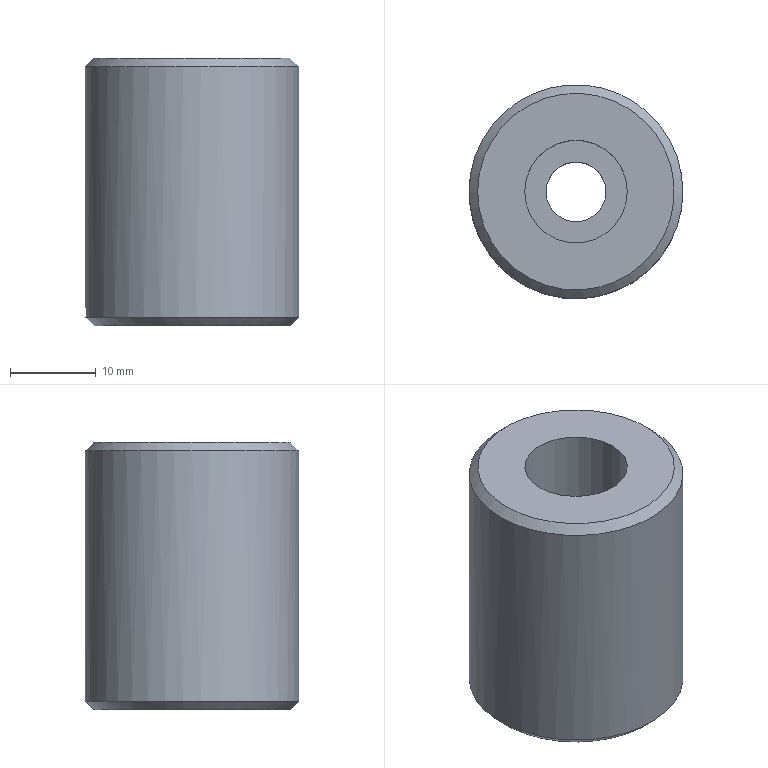Part | NX | features LIN_SOLID_COLOR 2 | 1 solid | 8 faces | box 25 x 25 x 31.3 mm | volume 13240 mm3 | plane 3 | cylinder 3 | cone 2 | commonest cylinder face diameters 7 x1 12 x1 25 x1
STEP:
#1=CARTESIAN_POINT('',(111.5,-150.,-31.5));
#2=VERTEX_POINT('',#1);
#3=CARTESIAN_POINT('',(100.,-150.,-31.5));
#4=DIRECTION('',(0.,0.,1.));
#5=DIRECTION('',(1.,0.,0.));
#6=AXIS2_PLACEMENT_3D('',#3,#4,#5);
#7=CIRCLE('',#6,11.5);
#8=EDGE_CURVE('',#2,#2,#7,.T.);
#9=ORIENTED_EDGE('',*,*,#8,.F.);
#10=EDGE_LOOP('',(#9));
#11=FACE_BOUND('',#10,.T.);
#12=CARTESIAN_POINT('',(96.5,-150.,-31.5));
#13=VERTEX_POINT('',#12);
#14=CARTESIAN_POINT('',(100.,-150.,-31.5));
#15=DIRECTION('',(0.,0.,-1.));
#16=DIRECTION('',(-1.,0.,0.));
#17=AXIS2_PLACEMENT_3D('',#14,#15,#16);
#18=CIRCLE('',#17,3.5);
#19=EDGE_CURVE('',#13,#13,#18,.T.);
#20=ORIENTED_EDGE('',*,*,#19,.F.);
#21=EDGE_LOOP('',(#20));
#22=FACE_BOUND('',#21,.T.);
#23=CARTESIAN_POINT('',(-237.,-10.,-31.5));
#24=DIRECTION('',(0.,0.,-1.));
#25=DIRECTION('',(1.,0.,0.));
#26=AXIS2_PLACEMENT_3D('',#23,#24,#25);
#27=PLANE('',#26);
#28=ADVANCED_FACE('',(#11,#22),#27,.T.);
#29=CARTESIAN_POINT('',(88.5,-150.,-0.2));
#30=VERTEX_POINT('',#29);
#31=CARTESIAN_POINT('',(100.,-150.,-0.2));
#32=DIRECTION('',(0.,0.,-1.));
#33=DIRECTION('',(-1.,0.,0.));
#34=AXIS2_PLACEMENT_3D('',#31,#32,#33);
#35=CIRCLE('',#34,11.5);
#36=EDGE_CURVE('',#30,#30,#35,.T.);
#37=ORIENTED_EDGE('',*,*,#36,.F.);
#38=EDGE_LOOP('',(#37));
#39=FACE_BOUND('',#38,.T.);
#40=CARTESIAN_POINT('',(106.,-150.,-0.2));
#41=VERTEX_POINT('',#40);
#42=CARTESIAN_POINT('',(100.,-150.,-0.2));
#43=DIRECTION('',(0.,0.,1.));
#44=DIRECTION('',(1.,0.,0.));
#45=AXIS2_PLACEMENT_3D('',#42,#43,#44);
#46=CIRCLE('',#45,6.);
#47=EDGE_CURVE('',#41,#41,#46,.F.);
#48=ORIENTED_EDGE('',*,*,#47,.T.);
#49=EDGE_LOOP('',(#48));
#50=FACE_BOUND('',#49,.T.);
#51=CARTESIAN_POINT('',(100.,-150.,-0.2));
#52=DIRECTION('',(0.,0.,1.));
#53=DIRECTION('',(-1.,0.,0.));
#54=AXIS2_PLACEMENT_3D('',#51,#52,#53);
#55=PLANE('',#54);
#56=ADVANCED_FACE('',(#39,#50),#55,.T.);
#57=CARTESIAN_POINT('',(112.5,-150.,-30.5));
#58=VERTEX_POINT('',#57);
#59=CARTESIAN_POINT('',(100.,-150.,-30.5));
#60=DIRECTION('',(0.,0.,1.));
#61=DIRECTION('',(1.,0.,0.));
#62=AXIS2_PLACEMENT_3D('',#59,#60,#61);
#63=CIRCLE('',#62,12.5);
#64=EDGE_CURVE('',#58,#58,#63,.F.);
#65=ORIENTED_EDGE('',*,*,#64,.F.);
#66=EDGE_LOOP('',(#65));
#67=FACE_BOUND('',#66,.T.);
#68=CARTESIAN_POINT('',(87.5,-150.,-1.2));
#69=VERTEX_POINT('',#68);
#70=CARTESIAN_POINT('',(100.,-150.,-1.2));
#71=DIRECTION('',(0.,0.,-1.));
#72=DIRECTION('',(-1.,0.,0.));
#73=AXIS2_PLACEMENT_3D('',#70,#71,#72);
#74=CIRCLE('',#73,12.5);
#75=EDGE_CURVE('',#69,#69,#74,.F.);
#76=ORIENTED_EDGE('',*,*,#75,.F.);
#77=EDGE_LOOP('',(#76));
#78=FACE_BOUND('',#77,.T.);
#79=CARTESIAN_POINT('',(100.,-150.,-1.5));
#80=DIRECTION('',(0.,0.,-1.));
#81=DIRECTION('',(1.,0.,0.));
#82=AXIS2_PLACEMENT_3D('',#79,#80,#81);
#83=CYLINDRICAL_SURFACE('',#82,12.5);
#84=ADVANCED_FACE('',(#67,#78),#83,.T.);
#85=CARTESIAN_POINT('',(96.5,-150.,-11.5));
#86=VERTEX_POINT('',#85);
#87=CARTESIAN_POINT('',(100.,-150.,-11.5));
#88=DIRECTION('',(0.,0.,-1.));
#89=DIRECTION('',(-1.,0.,0.));
#90=AXIS2_PLACEMENT_3D('',#87,#88,#89);
#91=CIRCLE('',#90,3.5);
#92=EDGE_CURVE('',#86,#86,#91,.T.);
#93=ORIENTED_EDGE('',*,*,#92,.F.);
#94=EDGE_LOOP('',(#93));
#95=FACE_BOUND('',#94,.T.);
#96=ORIENTED_EDGE('',*,*,#19,.T.);
#97=EDGE_LOOP('',(#96));
#98=FACE_BOUND('',#97,.T.);
#99=CARTESIAN_POINT('',(100.,-150.,-31.5));
#100=DIRECTION('',(0.,0.,1.));
#101=DIRECTION('',(-1.,0.,0.));
#102=AXIS2_PLACEMENT_3D('',#99,#100,#101);
#103=CYLINDRICAL_SURFACE('',#102,3.5);
#104=ADVANCED_FACE('',(#95,#98),#103,.F.);
#105=CARTESIAN_POINT('',(94.,-150.,-11.5));
#106=VERTEX_POINT('',#105);
#107=CARTESIAN_POINT('',(100.,-150.,-11.5));
#108=DIRECTION('',(0.,0.,-1.));
#109=DIRECTION('',(-1.,0.,0.));
#110=AXIS2_PLACEMENT_3D('',#107,#108,#109);
#111=CIRCLE('',#110,6.);
#112=EDGE_CURVE('',#106,#106,#111,.F.);
#113=ORIENTED_EDGE('',*,*,#112,.T.);
#114=EDGE_LOOP('',(#113));
#115=FACE_BOUND('',#114,.T.);
#116=ORIENTED_EDGE('',*,*,#92,.T.);
#117=EDGE_LOOP('',(#116));
#118=FACE_BOUND('',#117,.T.);
#119=CARTESIAN_POINT('',(100.,-150.,-11.5));
#120=DIRECTION('',(0.,0.,-1.));
#121=DIRECTION('',(1.,0.,0.));
#122=AXIS2_PLACEMENT_3D('',#119,#120,#121);
#123=PLANE('',#122);
#124=ADVANCED_FACE('',(#115,#118),#123,.F.);
#125=ORIENTED_EDGE('',*,*,#47,.F.);
#126=EDGE_LOOP('',(#125));
#127=FACE_BOUND('',#126,.T.);
#128=ORIENTED_EDGE('',*,*,#112,.F.);
#129=EDGE_LOOP('',(#128));
#130=FACE_BOUND('',#129,.T.);
#131=CARTESIAN_POINT('',(100.,-150.,-11.5));
#132=DIRECTION('',(0.,0.,1.));
#133=DIRECTION('',(-1.,0.,0.));
#134=AXIS2_PLACEMENT_3D('',#131,#132,#133);
#135=CYLINDRICAL_SURFACE('',#134,6.);
#136=ADVANCED_FACE('',(#127,#130),#135,.F.);
#137=ORIENTED_EDGE('',*,*,#64,.T.);
#138=EDGE_LOOP('',(#137));
#139=FACE_BOUND('',#138,.T.);
#140=ORIENTED_EDGE('',*,*,#8,.T.);
#141=EDGE_LOOP('',(#140));
#142=FACE_BOUND('',#141,.T.);
#143=CARTESIAN_POINT('',(100.,-150.,-31.5));
#144=DIRECTION('',(0.,0.,1.));
#145=DIRECTION('',(-1.,0.,0.));
#146=AXIS2_PLACEMENT_3D('',#143,#144,#145);
#147=CONICAL_SURFACE('',#146,11.5,0.7854);
#148=ADVANCED_FACE('',(#139,#142),#147,.T.);
#149=ORIENTED_EDGE('',*,*,#36,.T.);
#150=EDGE_LOOP('',(#149));
#151=FACE_BOUND('',#150,.T.);
#152=ORIENTED_EDGE('',*,*,#75,.T.);
#153=EDGE_LOOP('',(#152));
#154=FACE_BOUND('',#153,.T.);
#155=CARTESIAN_POINT('',(100.,-150.,-1.2));
#156=DIRECTION('',(0.,0.,-1.));
#157=DIRECTION('',(1.,0.,0.));
#158=AXIS2_PLACEMENT_3D('',#155,#156,#157);
#159=CONICAL_SURFACE('',#158,12.5,0.7854);
#160=ADVANCED_FACE('',(#151,#154),#159,.T.);
#161=CLOSED_SHELL('',(#28,#56,#84,#104,#124,#136,#148,#160));
#162=MANIFOLD_SOLID_BREP('',#161);
#163=(LENGTH_UNIT()NAMED_UNIT(*)SI_UNIT(.MILLI.,.METRE.));
#164=UNCERTAINTY_MEASURE_WITH_UNIT(LENGTH_MEASURE(0.00001),#163,'','');
#165=(NAMED_UNIT(*)PLANE_ANGLE_UNIT()SI_UNIT($,.RADIAN.));
#166=(NAMED_UNIT(*)SI_UNIT($,.STERADIAN.)SOLID_ANGLE_UNIT());
#167=(GEOMETRIC_REPRESENTATION_CONTEXT(3)GLOBAL_UNCERTAINTY_ASSIGNED_CONTEXT((#164))GLOBAL_UNIT_ASSIGNED_CONTEXT((#163,#165,#166))REPRESENTATION_CONTEXT('',''));
#168=ADVANCED_BREP_SHAPE_REPRESENTATION('',(#162),#167);